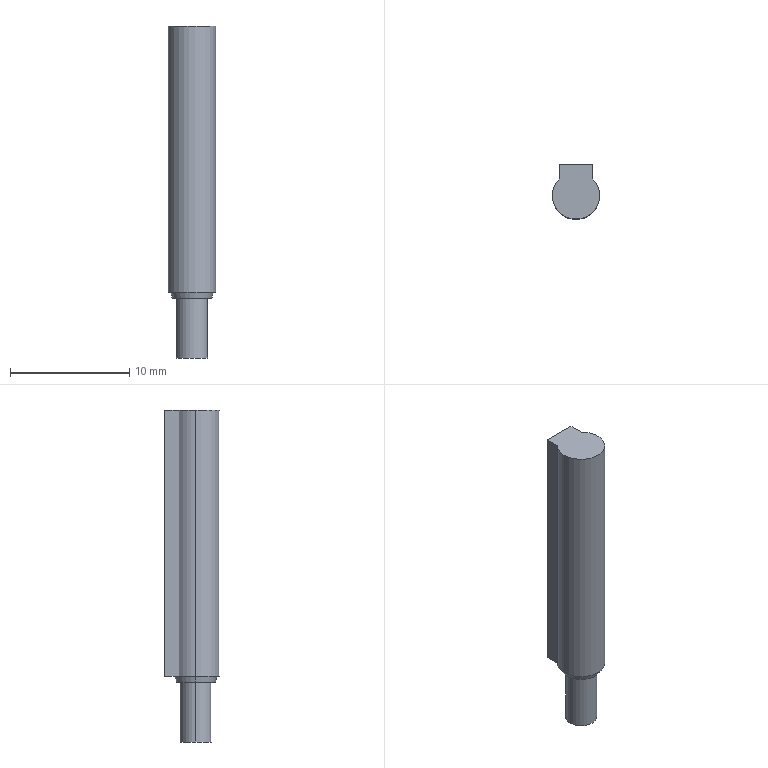Part | SolidWorks | features BaseBody 1 | 1 solid | 33 faces | box 3.95 x 4.575 x 27.8 mm | volume 349.99 mm3 | plane 18 | cylinder 13 | cone 2 | commonest cylinder face diameters 0.6 x4 3.95 x3 2 x2 2.5 x2 2.6 x2
STEP:
#1=CARTESIAN_POINT('',(-1.4,1.393,-22.3));
#2=VERTEX_POINT('',#1);
#3=CARTESIAN_POINT('',(-1.975,0.,-22.3));
#4=VERTEX_POINT('',#3);
#5=CARTESIAN_POINT('',(0.,0.,-22.3));
#6=DIRECTION('',(0.,0.,1.));
#7=DIRECTION('',(1.,0.,0.));
#8=AXIS2_PLACEMENT_3D('',#5,#6,#7);
#9=CIRCLE('',#8,1.975);
#10=EDGE_CURVE('',#2,#4,#9,.T.);
#11=ORIENTED_EDGE('',*,*,#10,.T.);
#12=CARTESIAN_POINT('',(-1.975,0.,0.));
#13=VERTEX_POINT('',#12);
#14=CARTESIAN_POINT('',(-1.975,0.,-22.3));
#15=DIRECTION('',(0.,0.,1.));
#16=VECTOR('',#15,1000.);
#17=LINE('',#14,#16);
#18=EDGE_CURVE('',#4,#13,#17,.T.);
#19=ORIENTED_EDGE('',*,*,#18,.T.);
#20=CARTESIAN_POINT('',(-1.4,1.393,0.));
#21=VERTEX_POINT('',#20);
#22=CARTESIAN_POINT('',(0.,0.,0.));
#23=DIRECTION('',(0.,0.,-1.));
#24=DIRECTION('',(1.,0.,0.));
#25=AXIS2_PLACEMENT_3D('',#22,#23,#24);
#26=CIRCLE('',#25,1.975);
#27=EDGE_CURVE('',#13,#21,#26,.T.);
#28=ORIENTED_EDGE('',*,*,#27,.T.);
#29=CARTESIAN_POINT('',(-1.4,1.393,-22.3));
#30=DIRECTION('',(0.,0.,-1.));
#31=VECTOR('',#30,1000.);
#32=LINE('',#29,#31);
#33=EDGE_CURVE('',#21,#2,#32,.T.);
#34=ORIENTED_EDGE('',*,*,#33,.T.);
#35=EDGE_LOOP('',(#11,#19,#28,#34));
#36=FACE_OUTER_BOUND('',#35,.T.);
#37=CARTESIAN_POINT('',(0.,0.,-22.3));
#38=DIRECTION('',(0.,0.,1.));
#39=DIRECTION('',(1.,0.,0.));
#40=AXIS2_PLACEMENT_3D('',#37,#38,#39);
#41=CYLINDRICAL_SURFACE('',#40,1.975);
#42=ADVANCED_FACE('',(#36),#41,.T.);
#43=ORIENTED_EDGE('',*,*,#18,.F.);
#44=CARTESIAN_POINT('',(1.975,0.,-22.3));
#45=VERTEX_POINT('',#44);
#46=CARTESIAN_POINT('',(0.,0.,-22.3));
#47=DIRECTION('',(0.,0.,1.));
#48=DIRECTION('',(1.,0.,0.));
#49=AXIS2_PLACEMENT_3D('',#46,#47,#48);
#50=CIRCLE('',#49,1.975);
#51=EDGE_CURVE('',#4,#45,#50,.T.);
#52=ORIENTED_EDGE('',*,*,#51,.T.);
#53=CARTESIAN_POINT('',(1.975,0.,0.));
#54=VERTEX_POINT('',#53);
#55=CARTESIAN_POINT('',(1.975,0.,-22.3));
#56=DIRECTION('',(0.,0.,1.));
#57=VECTOR('',#56,1000.);
#58=LINE('',#55,#57);
#59=EDGE_CURVE('',#45,#54,#58,.T.);
#60=ORIENTED_EDGE('',*,*,#59,.T.);
#61=CARTESIAN_POINT('',(0.,0.,0.));
#62=DIRECTION('',(0.,0.,-1.));
#63=DIRECTION('',(1.,0.,0.));
#64=AXIS2_PLACEMENT_3D('',#61,#62,#63);
#65=CIRCLE('',#64,1.975);
#66=EDGE_CURVE('',#54,#13,#65,.T.);
#67=ORIENTED_EDGE('',*,*,#66,.T.);
#68=EDGE_LOOP('',(#43,#52,#60,#67));
#69=FACE_OUTER_BOUND('',#68,.T.);
#70=CARTESIAN_POINT('',(0.,0.,-22.3));
#71=DIRECTION('',(0.,0.,1.));
#72=DIRECTION('',(1.,0.,0.));
#73=AXIS2_PLACEMENT_3D('',#70,#71,#72);
#74=CYLINDRICAL_SURFACE('',#73,1.975);
#75=ADVANCED_FACE('',(#69),#74,.T.);
#76=CARTESIAN_POINT('',(1.65,0.,-22.8));
#77=VERTEX_POINT('',#76);
#78=CARTESIAN_POINT('',(-1.65,0.,-22.8));
#79=VERTEX_POINT('',#78);
#80=CARTESIAN_POINT('',(0.,0.,-22.8));
#81=DIRECTION('',(0.,0.,1.));
#82=DIRECTION('',(1.,0.,0.));
#83=AXIS2_PLACEMENT_3D('',#80,#81,#82);
#84=CIRCLE('',#83,1.65);
#85=EDGE_CURVE('',#77,#79,#84,.T.);
#86=ORIENTED_EDGE('',*,*,#85,.T.);
#87=CARTESIAN_POINT('',(-1.784,0.,-22.3));
#88=VERTEX_POINT('',#87);
#89=CARTESIAN_POINT('',(-1.784,0.,-22.3));
#90=DIRECTION('',(-0.2588,0.,0.9659));
#91=VECTOR('',#90,1000.);
#92=LINE('',#89,#91);
#93=EDGE_CURVE('',#79,#88,#92,.T.);
#94=ORIENTED_EDGE('',*,*,#93,.T.);
#95=CARTESIAN_POINT('',(1.784,0.,-22.3));
#96=VERTEX_POINT('',#95);
#97=CARTESIAN_POINT('',(0.,0.,-22.3));
#98=DIRECTION('',(0.,0.,1.));
#99=DIRECTION('',(1.,0.,0.));
#100=AXIS2_PLACEMENT_3D('',#97,#98,#99);
#101=CIRCLE('',#100,1.784);
#102=EDGE_CURVE('',#96,#88,#101,.T.);
#103=ORIENTED_EDGE('',*,*,#102,.F.);
#104=CARTESIAN_POINT('',(1.784,0.,-22.3));
#105=DIRECTION('',(0.2588,0.,0.9659));
#106=VECTOR('',#105,1000.);
#107=LINE('',#104,#106);
#108=EDGE_CURVE('',#77,#96,#107,.T.);
#109=ORIENTED_EDGE('',*,*,#108,.F.);
#110=EDGE_LOOP('',(#86,#94,#103,#109));
#111=FACE_OUTER_BOUND('',#110,.T.);
#112=CARTESIAN_POINT('',(0.,0.,-22.3));
#113=DIRECTION('',(0.,0.,1.));
#114=DIRECTION('',(1.,0.,0.));
#115=AXIS2_PLACEMENT_3D('',#112,#113,#114);
#116=CONICAL_SURFACE('',#115,1.784,0.2618);
#117=ADVANCED_FACE('',(#111),#116,.T.);
#118=CARTESIAN_POINT('',(0.,1.1,-3.25));
#119=VERTEX_POINT('',#118);
#120=CARTESIAN_POINT('',(0.,1.1,-0.75));
#121=VERTEX_POINT('',#120);
#122=CARTESIAN_POINT('',(0.,1.1,-2.));
#123=DIRECTION('',(0.,1.,0.));
#124=DIRECTION('',(0.,0.,1.));
#125=AXIS2_PLACEMENT_3D('',#122,#123,#124);
#126=CIRCLE('',#125,1.25);
#127=EDGE_CURVE('',#119,#121,#126,.T.);
#128=ORIENTED_EDGE('',*,*,#127,.F.);
#129=CARTESIAN_POINT('',(0.,2.6,-3.25));
#130=VERTEX_POINT('',#129);
#131=CARTESIAN_POINT('',(0.,1.1,-3.25));
#132=DIRECTION('',(0.,1.,0.));
#133=VECTOR('',#132,1000.);
#134=LINE('',#131,#133);
#135=EDGE_CURVE('',#119,#130,#134,.T.);
#136=ORIENTED_EDGE('',*,*,#135,.T.);
#137=CARTESIAN_POINT('',(0.,2.6,-0.75));
#138=VERTEX_POINT('',#137);
#139=CARTESIAN_POINT('',(0.,2.6,-2.));
#140=DIRECTION('',(0.,1.,0.));
#141=DIRECTION('',(0.,0.,1.));
#142=AXIS2_PLACEMENT_3D('',#139,#140,#141);
#143=CIRCLE('',#142,1.25);
#144=EDGE_CURVE('',#130,#138,#143,.T.);
#145=ORIENTED_EDGE('',*,*,#144,.T.);
#146=CARTESIAN_POINT('',(0.,1.1,-0.75));
#147=DIRECTION('',(0.,1.,0.));
#148=VECTOR('',#147,1000.);
#149=LINE('',#146,#148);
#150=EDGE_CURVE('',#121,#138,#149,.T.);
#151=ORIENTED_EDGE('',*,*,#150,.F.);
#152=EDGE_LOOP('',(#128,#136,#145,#151));
#153=FACE_OUTER_BOUND('',#152,.T.);
#154=CARTESIAN_POINT('',(0.,1.1,-2.));
#155=DIRECTION('',(0.,1.,0.));
#156=DIRECTION('',(0.,0.,1.));
#157=AXIS2_PLACEMENT_3D('',#154,#155,#156);
#158=CYLINDRICAL_SURFACE('',#157,1.25);
#159=ADVANCED_FACE('',(#153),#158,.F.);
#160=CARTESIAN_POINT('',(1.3,0.,-27.8));
#161=VERTEX_POINT('',#160);
#162=CARTESIAN_POINT('',(-1.3,0.,-27.8));
#163=VERTEX_POINT('',#162);
#164=CARTESIAN_POINT('',(0.,0.,-27.8));
#165=DIRECTION('',(0.,0.,1.));
#166=DIRECTION('',(1.,0.,0.));
#167=AXIS2_PLACEMENT_3D('',#164,#165,#166);
#168=CIRCLE('',#167,1.3);
#169=EDGE_CURVE('',#161,#163,#168,.T.);
#170=ORIENTED_EDGE('',*,*,#169,.T.);
#171=CARTESIAN_POINT('',(-1.3,0.,-22.8));
#172=VERTEX_POINT('',#171);
#173=CARTESIAN_POINT('',(-1.3,0.,-27.8));
#174=DIRECTION('',(0.,0.,1.));
#175=VECTOR('',#174,1000.);
#176=LINE('',#173,#175);
#177=EDGE_CURVE('',#163,#172,#176,.T.);
#178=ORIENTED_EDGE('',*,*,#177,.T.);
#179=CARTESIAN_POINT('',(1.3,0.,-22.8));
#180=VERTEX_POINT('',#179);
#181=CARTESIAN_POINT('',(0.,0.,-22.8));
#182=DIRECTION('',(0.,0.,-1.));
#183=DIRECTION('',(1.,0.,0.));
#184=AXIS2_PLACEMENT_3D('',#181,#182,#183);
#185=CIRCLE('',#184,1.3);
#186=EDGE_CURVE('',#172,#180,#185,.T.);
#187=ORIENTED_EDGE('',*,*,#186,.T.);
#188=CARTESIAN_POINT('',(1.3,0.,-27.8));
#189=DIRECTION('',(0.,0.,1.));
#190=VECTOR('',#189,1000.);
#191=LINE('',#188,#190);
#192=EDGE_CURVE('',#161,#180,#191,.T.);
#193=ORIENTED_EDGE('',*,*,#192,.F.);
#194=EDGE_LOOP('',(#170,#178,#187,#193));
#195=FACE_OUTER_BOUND('',#194,.T.);
#196=CARTESIAN_POINT('',(0.,0.,-27.8));
#197=DIRECTION('',(0.,0.,1.));
#198=DIRECTION('',(1.,0.,0.));
#199=AXIS2_PLACEMENT_3D('',#196,#197,#198);
#200=CYLINDRICAL_SURFACE('',#199,1.3);
#201=ADVANCED_FACE('',(#195),#200,.T.);
#202=CARTESIAN_POINT('',(0.,1.1,-3.));
#203=VERTEX_POINT('',#202);
#204=CARTESIAN_POINT('',(0.,1.1,-1.));
#205=VERTEX_POINT('',#204);
#206=CARTESIAN_POINT('',(0.,1.1,-2.));
#207=DIRECTION('',(0.,-1.,0.));
#208=DIRECTION('',(0.,0.,1.));
#209=AXIS2_PLACEMENT_3D('',#206,#207,#208);
#210=CIRCLE('',#209,1.);
#211=EDGE_CURVE('',#203,#205,#210,.T.);
#212=ORIENTED_EDGE('',*,*,#211,.F.);
#213=CARTESIAN_POINT('',(0.,2.6,-3.));
#214=VERTEX_POINT('',#213);
#215=CARTESIAN_POINT('',(0.,1.1,-3.));
#216=DIRECTION('',(0.,1.,0.));
#217=VECTOR('',#216,1000.);
#218=LINE('',#215,#217);
#219=EDGE_CURVE('',#203,#214,#218,.T.);
#220=ORIENTED_EDGE('',*,*,#219,.T.);
#221=CARTESIAN_POINT('',(0.8867,2.6,-1.538));
#222=VERTEX_POINT('',#221);
#223=CARTESIAN_POINT('',(0.,2.6,-2.));
#224=DIRECTION('',(0.,-1.,0.));
#225=DIRECTION('',(0.,0.,1.));
#226=AXIS2_PLACEMENT_3D('',#223,#224,#225);
#227=CIRCLE('',#226,1.);
#228=EDGE_CURVE('',#214,#222,#227,.T.);
#229=ORIENTED_EDGE('',*,*,#228,.T.);
#230=CARTESIAN_POINT('',(0.8867,1.6,-1.538));
#231=VERTEX_POINT('',#230);
#232=CARTESIAN_POINT('',(0.8867,1.6,-1.538));
#233=DIRECTION('',(0.,-1.,0.));
#234=VECTOR('',#233,1000.);
#235=LINE('',#232,#234);
#236=EDGE_CURVE('',#222,#231,#235,.T.);
#237=ORIENTED_EDGE('',*,*,#236,.T.);
#238=CARTESIAN_POINT('',(0.4624,1.6,-1.113));
#239=VERTEX_POINT('',#238);
#240=CARTESIAN_POINT('',(0.,1.6,-2.));
#241=DIRECTION('',(0.,1.,0.));
#242=DIRECTION('',(0.,0.,1.));
#243=AXIS2_PLACEMENT_3D('',#240,#241,#242);
#244=CIRCLE('',#243,1.);
#245=EDGE_CURVE('',#239,#231,#244,.T.);
#246=ORIENTED_EDGE('',*,*,#245,.F.);
#247=CARTESIAN_POINT('',(0.4624,2.6,-1.113));
#248=VERTEX_POINT('',#247);
#249=CARTESIAN_POINT('',(0.4624,1.6,-1.113));
#250=DIRECTION('',(0.,1.,0.));
#251=VECTOR('',#250,1000.);
#252=LINE('',#249,#251);
#253=EDGE_CURVE('',#239,#248,#252,.T.);
#254=ORIENTED_EDGE('',*,*,#253,.T.);
#255=CARTESIAN_POINT('',(0.,2.6,-1.));
#256=VERTEX_POINT('',#255);
#257=CARTESIAN_POINT('',(0.,2.6,-2.));
#258=DIRECTION('',(0.,-1.,0.));
#259=DIRECTION('',(0.,0.,1.));
#260=AXIS2_PLACEMENT_3D('',#257,#258,#259);
#261=CIRCLE('',#260,1.);
#262=EDGE_CURVE('',#248,#256,#261,.T.);
#263=ORIENTED_EDGE('',*,*,#262,.T.);
#264=CARTESIAN_POINT('',(0.,1.1,-1.));
#265=DIRECTION('',(0.,1.,0.));
#266=VECTOR('',#265,1000.);
#267=LINE('',#264,#266);
#268=EDGE_CURVE('',#205,#256,#267,.T.);
#269=ORIENTED_EDGE('',*,*,#268,.F.);
#270=EDGE_LOOP('',(#212,#220,#229,#237,#246,#254,#263,#269));
#271=FACE_OUTER_BOUND('',#270,.T.);
#272=CARTESIAN_POINT('',(0.,1.1,-2.));
#273=DIRECTION('',(0.,1.,0.));
#274=DIRECTION('',(0.,0.,1.));
#275=AXIS2_PLACEMENT_3D('',#272,#273,#274);
#276=CYLINDRICAL_SURFACE('',#275,1.);
#277=ADVANCED_FACE('',(#271),#276,.T.);
#278=ORIENTED_EDGE('',*,*,#59,.F.);
#279=CARTESIAN_POINT('',(1.4,1.393,-22.3));
#280=VERTEX_POINT('',#279);
#281=CARTESIAN_POINT('',(0.,0.,-22.3));
#282=DIRECTION('',(0.,0.,1.));
#283=DIRECTION('',(1.,0.,0.));
#284=AXIS2_PLACEMENT_3D('',#281,#282,#283);
#285=CIRCLE('',#284,1.975);
#286=EDGE_CURVE('',#45,#280,#285,.T.);
#287=ORIENTED_EDGE('',*,*,#286,.T.);
#288=CARTESIAN_POINT('',(1.4,1.393,0.));
#289=VERTEX_POINT('',#288);
#290=CARTESIAN_POINT('',(1.4,1.393,-22.3));
#291=DIRECTION('',(0.,0.,1.));
#292=VECTOR('',#291,1000.);
#293=LINE('',#290,#292);
#294=EDGE_CURVE('',#280,#289,#293,.T.);
#295=ORIENTED_EDGE('',*,*,#294,.T.);
#296=CARTESIAN_POINT('',(0.,0.,0.));
#297=DIRECTION('',(0.,0.,-1.));
#298=DIRECTION('',(1.,0.,0.));
#299=AXIS2_PLACEMENT_3D('',#296,#297,#298);
#300=CIRCLE('',#299,1.975);
#301=EDGE_CURVE('',#289,#54,#300,.T.);
#302=ORIENTED_EDGE('',*,*,#301,.T.);
#303=EDGE_LOOP('',(#278,#287,#295,#302));
#304=FACE_OUTER_BOUND('',#303,.T.);
#305=CARTESIAN_POINT('',(0.,0.,-22.3));
#306=DIRECTION('',(0.,0.,1.));
#307=DIRECTION('',(1.,0.,0.));
#308=AXIS2_PLACEMENT_3D('',#305,#306,#307);
#309=CYLINDRICAL_SURFACE('',#308,1.975);
#310=ADVANCED_FACE('',(#304),#309,.T.);
#311=ORIENTED_EDGE('',*,*,#294,.F.);
#312=CARTESIAN_POINT('',(1.4,2.6,-22.3));
#313=VERTEX_POINT('',#312);
#314=CARTESIAN_POINT('',(1.4,2.6,-22.3));
#315=DIRECTION('',(0.,-1.,0.));
#316=VECTOR('',#315,1000.);
#317=LINE('',#314,#316);
#318=EDGE_CURVE('',#313,#280,#317,.T.);
#319=ORIENTED_EDGE('',*,*,#318,.F.);
#320=CARTESIAN_POINT('',(1.4,2.6,0.));
#321=VERTEX_POINT('',#320);
#322=CARTESIAN_POINT('',(1.4,2.6,-22.3));
#323=DIRECTION('',(0.,0.,-1.));
#324=VECTOR('',#323,1000.);
#325=LINE('',#322,#324);
#326=EDGE_CURVE('',#321,#313,#325,.T.);
#327=ORIENTED_EDGE('',*,*,#326,.F.);
#328=CARTESIAN_POINT('',(1.4,2.6,0.));
#329=DIRECTION('',(0.,1.,0.));
#330=VECTOR('',#329,1000.);
#331=LINE('',#328,#330);
#332=EDGE_CURVE('',#289,#321,#331,.T.);
#333=ORIENTED_EDGE('',*,*,#332,.F.);
#334=EDGE_LOOP('',(#311,#319,#327,#333));
#335=FACE_OUTER_BOUND('',#334,.T.);
#336=CARTESIAN_POINT('',(1.4,2.6,-22.3));
#337=DIRECTION('',(-1.,0.,0.));
#338=DIRECTION('',(0.,0.,1.));
#339=AXIS2_PLACEMENT_3D('',#336,#337,#338);
#340=PLANE('',#339);
#341=ADVANCED_FACE('',(#335),#340,.F.);
#342=CARTESIAN_POINT('',(-1.4,2.6,-22.3));
#343=VERTEX_POINT('',#342);
#344=CARTESIAN_POINT('',(-1.4,0.,-22.3));
#345=DIRECTION('',(0.,1.,0.));
#346=VECTOR('',#345,1000.);
#347=LINE('',#344,#346);
#348=EDGE_CURVE('',#2,#343,#347,.T.);
#349=ORIENTED_EDGE('',*,*,#348,.T.);
#350=CARTESIAN_POINT('',(0.,2.6,-22.3));
#351=DIRECTION('',(1.,0.,0.));
#352=VECTOR('',#351,1000.);
#353=LINE('',#350,#352);
#354=EDGE_CURVE('',#343,#313,#353,.T.);
#355=ORIENTED_EDGE('',*,*,#354,.T.);
#356=ORIENTED_EDGE('',*,*,#318,.T.);
#357=ORIENTED_EDGE('',*,*,#286,.F.);
#358=ORIENTED_EDGE('',*,*,#51,.F.);
#359=ORIENTED_EDGE('',*,*,#10,.F.);
#360=EDGE_LOOP('',(#349,#355,#356,#357,#358,#359));
#361=FACE_OUTER_BOUND('',#360,.T.);
#362=ORIENTED_EDGE('',*,*,#102,.T.);
#363=CARTESIAN_POINT('',(0.,0.,-22.3));
#364=DIRECTION('',(0.,0.,1.));
#365=DIRECTION('',(1.,0.,0.));
#366=AXIS2_PLACEMENT_3D('',#363,#364,#365);
#367=CIRCLE('',#366,1.784);
#368=EDGE_CURVE('',#88,#96,#367,.T.);
#369=ORIENTED_EDGE('',*,*,#368,.T.);
#370=EDGE_LOOP('',(#362,#369));
#371=FACE_BOUND('',#370,.T.);
#372=CARTESIAN_POINT('',(0.,0.,-22.3));
#373=DIRECTION('',(0.,0.,-1.));
#374=DIRECTION('',(-1.,0.,0.));
#375=AXIS2_PLACEMENT_3D('',#372,#373,#374);
#376=PLANE('',#375);
#377=ADVANCED_FACE('',(#361,#371),#376,.T.);
#378=CARTESIAN_POINT('',(-1.4,2.6,0.));
#379=VERTEX_POINT('',#378);
#380=CARTESIAN_POINT('',(-1.4,2.6,-22.3));
#381=DIRECTION('',(0.,0.,1.));
#382=VECTOR('',#381,1000.);
#383=LINE('',#380,#382);
#384=EDGE_CURVE('',#343,#379,#383,.T.);
#385=ORIENTED_EDGE('',*,*,#384,.F.);
#386=ORIENTED_EDGE('',*,*,#348,.F.);
#387=ORIENTED_EDGE('',*,*,#33,.F.);
#388=CARTESIAN_POINT('',(-1.4,1.393,0.));
#389=DIRECTION('',(0.,-1.,0.));
#390=VECTOR('',#389,1000.);
#391=LINE('',#388,#390);
#392=EDGE_CURVE('',#379,#21,#391,.T.);
#393=ORIENTED_EDGE('',*,*,#392,.F.);
#394=EDGE_LOOP('',(#385,#386,#387,#393));
#395=FACE_OUTER_BOUND('',#394,.T.);
#396=CARTESIAN_POINT('',(-1.4,1.393,-22.3));
#397=DIRECTION('',(1.,0.,0.));
#398=DIRECTION('',(0.,0.,-1.));
#399=AXIS2_PLACEMENT_3D('',#396,#397,#398);
#400=PLANE('',#399);
#401=ADVANCED_FACE('',(#395),#400,.F.);
#402=CARTESIAN_POINT('',(0.,2.6,0.));
#403=DIRECTION('',(1.,0.,0.));
#404=VECTOR('',#403,1000.);
#405=LINE('',#402,#404);
#406=EDGE_CURVE('',#379,#321,#405,.T.);
#407=ORIENTED_EDGE('',*,*,#406,.F.);
#408=ORIENTED_EDGE('',*,*,#392,.T.);
#409=ORIENTED_EDGE('',*,*,#27,.F.);
#410=ORIENTED_EDGE('',*,*,#66,.F.);
#411=ORIENTED_EDGE('',*,*,#301,.F.);
#412=ORIENTED_EDGE('',*,*,#332,.T.);
#413=EDGE_LOOP('',(#407,#408,#409,#410,#411,#412));
#414=FACE_OUTER_BOUND('',#413,.T.);
#415=CARTESIAN_POINT('',(0.,0.,0.));
#416=DIRECTION('',(0.,0.,-1.));
#417=DIRECTION('',(-1.,0.,0.));
#418=AXIS2_PLACEMENT_3D('',#415,#416,#417);
#419=PLANE('',#418);
#420=ADVANCED_FACE('',(#414),#419,.F.);
#421=ORIENTED_EDGE('',*,*,#326,.T.);
#422=ORIENTED_EDGE('',*,*,#354,.F.);
#423=ORIENTED_EDGE('',*,*,#384,.T.);
#424=ORIENTED_EDGE('',*,*,#406,.T.);
#425=EDGE_LOOP('',(#421,#422,#423,#424));
#426=FACE_OUTER_BOUND('',#425,.T.);
#427=CARTESIAN_POINT('',(0.,2.6,-2.));
#428=DIRECTION('',(0.,1.,0.));
#429=DIRECTION('',(0.,0.,1.));
#430=AXIS2_PLACEMENT_3D('',#427,#428,#429);
#431=CIRCLE('',#430,1.25);
#432=EDGE_CURVE('',#138,#130,#431,.T.);
#433=ORIENTED_EDGE('',*,*,#432,.F.);
#434=ORIENTED_EDGE('',*,*,#144,.F.);
#435=EDGE_LOOP('',(#433,#434));
#436=FACE_BOUND('',#435,.T.);
#437=CARTESIAN_POINT('',(-0.8,2.6,-8.3));
#438=VERTEX_POINT('',#437);
#439=CARTESIAN_POINT('',(-0.5,2.6,-8.));
#440=VERTEX_POINT('',#439);
#441=CARTESIAN_POINT('',(-0.5,2.6,-8.3));
#442=DIRECTION('',(0.,1.,0.));
#443=DIRECTION('',(0.,0.,1.));
#444=AXIS2_PLACEMENT_3D('',#441,#442,#443);
#445=CIRCLE('',#444,0.3);
#446=EDGE_CURVE('',#438,#440,#445,.T.);
#447=ORIENTED_EDGE('',*,*,#446,.F.);
#448=CARTESIAN_POINT('',(-0.8,2.6,-10.7));
#449=VERTEX_POINT('',#448);
#450=CARTESIAN_POINT('',(-0.8,2.6,-22.3));
#451=DIRECTION('',(0.,0.,1.));
#452=VECTOR('',#451,1000.);
#453=LINE('',#450,#452);
#454=EDGE_CURVE('',#449,#438,#453,.T.);
#455=ORIENTED_EDGE('',*,*,#454,.F.);
#456=CARTESIAN_POINT('',(-0.5,2.6,-11.));
#457=VERTEX_POINT('',#456);
#458=CARTESIAN_POINT('',(-0.5,2.6,-10.7));
#459=DIRECTION('',(0.,1.,0.));
#460=DIRECTION('',(0.,0.,1.));
#461=AXIS2_PLACEMENT_3D('',#458,#459,#460);
#462=CIRCLE('',#461,0.3);
#463=EDGE_CURVE('',#457,#449,#462,.T.);
#464=ORIENTED_EDGE('',*,*,#463,.F.);
#465=CARTESIAN_POINT('',(0.5,2.6,-11.));
#466=VERTEX_POINT('',#465);
#467=CARTESIAN_POINT('',(-1.4,2.6,-11.));
#468=DIRECTION('',(-1.,0.,0.));
#469=VECTOR('',#468,1000.);
#470=LINE('',#467,#469);
#471=EDGE_CURVE('',#466,#457,#470,.T.);
#472=ORIENTED_EDGE('',*,*,#471,.F.);
#473=CARTESIAN_POINT('',(0.8,2.6,-10.7));
#474=VERTEX_POINT('',#473);
#475=CARTESIAN_POINT('',(0.5,2.6,-10.7));
#476=DIRECTION('',(0.,1.,0.));
#477=DIRECTION('',(0.,0.,1.));
#478=AXIS2_PLACEMENT_3D('',#475,#476,#477);
#479=CIRCLE('',#478,0.3);
#480=EDGE_CURVE('',#474,#466,#479,.T.);
#481=ORIENTED_EDGE('',*,*,#480,.F.);
#482=CARTESIAN_POINT('',(0.8,2.6,-8.3));
#483=VERTEX_POINT('',#482);
#484=CARTESIAN_POINT('',(0.8,2.6,-22.3));
#485=DIRECTION('',(0.,0.,-1.));
#486=VECTOR('',#485,1000.);
#487=LINE('',#484,#486);
#488=EDGE_CURVE('',#483,#474,#487,.T.);
#489=ORIENTED_EDGE('',*,*,#488,.F.);
#490=CARTESIAN_POINT('',(0.5,2.6,-8.));
#491=VERTEX_POINT('',#490);
#492=CARTESIAN_POINT('',(0.5,2.6,-8.3));
#493=DIRECTION('',(0.,1.,0.));
#494=DIRECTION('',(0.,0.,1.));
#495=AXIS2_PLACEMENT_3D('',#492,#493,#494);
#496=CIRCLE('',#495,0.3);
#497=EDGE_CURVE('',#491,#483,#496,.T.);
#498=ORIENTED_EDGE('',*,*,#497,.F.);
#499=CARTESIAN_POINT('',(-1.4,2.6,-8.));
#500=DIRECTION('',(1.,0.,0.));
#501=VECTOR('',#500,1000.);
#502=LINE('',#499,#501);
#503=EDGE_CURVE('',#440,#491,#502,.T.);
#504=ORIENTED_EDGE('',*,*,#503,.F.);
#505=EDGE_LOOP('',(#447,#455,#464,#472,#481,#489,#498,#504));
#506=FACE_BOUND('',#505,.T.);
#507=CARTESIAN_POINT('',(-1.4,2.6,-22.3));
#508=DIRECTION('',(0.,-1.,0.));
#509=DIRECTION('',(0.,0.,-1.));
#510=AXIS2_PLACEMENT_3D('',#507,#508,#509);
#511=PLANE('',#510);
#512=ADVANCED_FACE('',(#426,#436,#506),#511,.F.);
#513=ORIENTED_EDGE('',*,*,#93,.F.);
#514=CARTESIAN_POINT('',(0.,0.,-22.8));
#515=DIRECTION('',(0.,0.,1.));
#516=DIRECTION('',(1.,0.,0.));
#517=AXIS2_PLACEMENT_3D('',#514,#515,#516);
#518=CIRCLE('',#517,1.65);
#519=EDGE_CURVE('',#79,#77,#518,.T.);
#520=ORIENTED_EDGE('',*,*,#519,.T.);
#521=ORIENTED_EDGE('',*,*,#108,.T.);
#522=ORIENTED_EDGE('',*,*,#368,.F.);
#523=EDGE_LOOP('',(#513,#520,#521,#522));
#524=FACE_OUTER_BOUND('',#523,.T.);
#525=CARTESIAN_POINT('',(0.,0.,-22.3));
#526=DIRECTION('',(0.,0.,1.));
#527=DIRECTION('',(1.,0.,0.));
#528=AXIS2_PLACEMENT_3D('',#525,#526,#527);
#529=CONICAL_SURFACE('',#528,1.784,0.2618);
#530=ADVANCED_FACE('',(#524),#529,.T.);
#531=ORIENTED_EDGE('',*,*,#135,.F.);
#532=CARTESIAN_POINT('',(0.,1.1,-2.));
#533=DIRECTION('',(0.,1.,0.));
#534=DIRECTION('',(0.,0.,1.));
#535=AXIS2_PLACEMENT_3D('',#532,#533,#534);
#536=CIRCLE('',#535,1.25);
#537=EDGE_CURVE('',#121,#119,#536,.T.);
#538=ORIENTED_EDGE('',*,*,#537,.F.);
#539=ORIENTED_EDGE('',*,*,#150,.T.);
#540=ORIENTED_EDGE('',*,*,#432,.T.);
#541=EDGE_LOOP('',(#531,#538,#539,#540));
#542=FACE_OUTER_BOUND('',#541,.T.);
#543=CARTESIAN_POINT('',(0.,1.1,-2.));
#544=DIRECTION('',(0.,1.,0.));
#545=DIRECTION('',(0.,0.,1.));
#546=AXIS2_PLACEMENT_3D('',#543,#544,#545);
#547=CYLINDRICAL_SURFACE('',#546,1.25);
#548=ADVANCED_FACE('',(#542),#547,.F.);
#549=CARTESIAN_POINT('',(0.5,2.4,-8.));
#550=VERTEX_POINT('',#549);
#551=CARTESIAN_POINT('',(0.5,2.4,-8.));
#552=DIRECTION('',(0.,1.,0.));
#553=VECTOR('',#552,1000.);
#554=LINE('',#551,#553);
#555=EDGE_CURVE('',#550,#491,#554,.T.);
#556=ORIENTED_EDGE('',*,*,#555,.F.);
#557=CARTESIAN_POINT('',(-0.5,2.4,-8.));
#558=VERTEX_POINT('',#557);
#559=CARTESIAN_POINT('',(-0.5,2.4,-8.));
#560=DIRECTION('',(1.,0.,0.));
#561=VECTOR('',#560,1000.);
#562=LINE('',#559,#561);
#563=EDGE_CURVE('',#558,#550,#562,.T.);
#564=ORIENTED_EDGE('',*,*,#563,.F.);
#565=CARTESIAN_POINT('',(-0.5,2.4,-8.));
#566=DIRECTION('',(0.,-1.,0.));
#567=VECTOR('',#566,1000.);
#568=LINE('',#565,#567);
#569=EDGE_CURVE('',#440,#558,#568,.T.);
#570=ORIENTED_EDGE('',*,*,#569,.F.);
#571=ORIENTED_EDGE('',*,*,#503,.T.);
#572=EDGE_LOOP('',(#556,#564,#570,#571));
#573=FACE_OUTER_BOUND('',#572,.T.);
#574=CARTESIAN_POINT('',(-0.5,2.4,-8.));
#575=DIRECTION('',(0.,0.,1.));
#576=DIRECTION('',(1.,0.,0.));
#577=AXIS2_PLACEMENT_3D('',#574,#575,#576);
#578=PLANE('',#577);
#579=ADVANCED_FACE('',(#573),#578,.F.);
#580=ORIENTED_EDGE('',*,*,#569,.T.);
#581=CARTESIAN_POINT('',(-0.8,2.4,-8.3));
#582=VERTEX_POINT('',#581);
#583=CARTESIAN_POINT('',(-0.5,2.4,-8.3));
#584=DIRECTION('',(0.,1.,0.));
#585=DIRECTION('',(0.,0.,1.));
#586=AXIS2_PLACEMENT_3D('',#583,#584,#585);
#587=CIRCLE('',#586,0.3);
#588=EDGE_CURVE('',#582,#558,#587,.T.);
#589=ORIENTED_EDGE('',*,*,#588,.F.);
#590=CARTESIAN_POINT('',(-0.8,2.4,-8.3));
#591=DIRECTION('',(0.,-1.,0.));
#592=VECTOR('',#591,1000.);
#593=LINE('',#590,#592);
#594=EDGE_CURVE('',#438,#582,#593,.T.);
#595=ORIENTED_EDGE('',*,*,#594,.F.);
#596=ORIENTED_EDGE('',*,*,#446,.T.);
#597=EDGE_LOOP('',(#580,#589,#595,#596));
#598=FACE_OUTER_BOUND('',#597,.T.);
#599=CARTESIAN_POINT('',(-0.5,2.4,-8.3));
#600=DIRECTION('',(0.,1.,0.));
#601=DIRECTION('',(0.,0.,1.));
#602=AXIS2_PLACEMENT_3D('',#599,#600,#601);
#603=CYLINDRICAL_SURFACE('',#602,0.3);
#604=ADVANCED_FACE('',(#598),#603,.F.);
#605=ORIENTED_EDGE('',*,*,#594,.T.);
#606=CARTESIAN_POINT('',(-0.8,2.4,-10.7));
#607=VERTEX_POINT('',#606);
#608=CARTESIAN_POINT('',(-0.8,2.4,-10.7));
#609=DIRECTION('',(0.,0.,1.));
#610=VECTOR('',#609,1000.);
#611=LINE('',#608,#610);
#612=EDGE_CURVE('',#607,#582,#611,.T.);
#613=ORIENTED_EDGE('',*,*,#612,.F.);
#614=CARTESIAN_POINT('',(-0.8,2.4,-10.7));
#615=DIRECTION('',(0.,-1.,0.));
#616=VECTOR('',#615,1000.);
#617=LINE('',#614,#616);
#618=EDGE_CURVE('',#449,#607,#617,.T.);
#619=ORIENTED_EDGE('',*,*,#618,.F.);
#620=ORIENTED_EDGE('',*,*,#454,.T.);
#621=EDGE_LOOP('',(#605,#613,#619,#620));
#622=FACE_OUTER_BOUND('',#621,.T.);
#623=CARTESIAN_POINT('',(-0.8,2.4,-10.7));
#624=DIRECTION('',(-1.,0.,0.));
#625=DIRECTION('',(0.,0.,1.));
#626=AXIS2_PLACEMENT_3D('',#623,#624,#625);
#627=PLANE('',#626);
#628=ADVANCED_FACE('',(#622),#627,.F.);
#629=ORIENTED_EDGE('',*,*,#618,.T.);
#630=CARTESIAN_POINT('',(-0.5,2.4,-11.));
#631=VERTEX_POINT('',#630);
#632=CARTESIAN_POINT('',(-0.5,2.4,-10.7));
#633=DIRECTION('',(0.,1.,0.));
#634=DIRECTION('',(0.,0.,1.));
#635=AXIS2_PLACEMENT_3D('',#632,#633,#634);
#636=CIRCLE('',#635,0.3);
#637=EDGE_CURVE('',#631,#607,#636,.T.);
#638=ORIENTED_EDGE('',*,*,#637,.F.);
#639=CARTESIAN_POINT('',(-0.5,2.4,-11.));
#640=DIRECTION('',(0.,-1.,0.));
#641=VECTOR('',#640,1000.);
#642=LINE('',#639,#641);
#643=EDGE_CURVE('',#457,#631,#642,.T.);
#644=ORIENTED_EDGE('',*,*,#643,.F.);
#645=ORIENTED_EDGE('',*,*,#463,.T.);
#646=EDGE_LOOP('',(#629,#638,#644,#645));
#647=FACE_OUTER_BOUND('',#646,.T.);
#648=CARTESIAN_POINT('',(-0.5,2.4,-10.7));
#649=DIRECTION('',(0.,1.,0.));
#650=DIRECTION('',(0.,0.,1.));
#651=AXIS2_PLACEMENT_3D('',#648,#649,#650);
#652=CYLINDRICAL_SURFACE('',#651,0.3);
#653=ADVANCED_FACE('',(#647),#652,.F.);
#654=ORIENTED_EDGE('',*,*,#643,.T.);
#655=CARTESIAN_POINT('',(0.5,2.4,-11.));
#656=VERTEX_POINT('',#655);
#657=CARTESIAN_POINT('',(0.5,2.4,-11.));
#658=DIRECTION('',(-1.,0.,0.));
#659=VECTOR('',#658,1000.);
#660=LINE('',#657,#659);
#661=EDGE_CURVE('',#656,#631,#660,.T.);
#662=ORIENTED_EDGE('',*,*,#661,.F.);
#663=CARTESIAN_POINT('',(0.5,2.4,-11.));
#664=DIRECTION('',(0.,-1.,0.));
#665=VECTOR('',#664,1000.);
#666=LINE('',#663,#665);
#667=EDGE_CURVE('',#466,#656,#666,.T.);
#668=ORIENTED_EDGE('',*,*,#667,.F.);
#669=ORIENTED_EDGE('',*,*,#471,.T.);
#670=EDGE_LOOP('',(#654,#662,#668,#669));
#671=FACE_OUTER_BOUND('',#670,.T.);
#672=CARTESIAN_POINT('',(0.5,2.4,-11.));
#673=DIRECTION('',(0.,0.,-1.));
#674=DIRECTION('',(-1.,0.,0.));
#675=AXIS2_PLACEMENT_3D('',#672,#673,#674);
#676=PLANE('',#675);
#677=ADVANCED_FACE('',(#671),#676,.F.);
#678=ORIENTED_EDGE('',*,*,#667,.T.);
#679=CARTESIAN_POINT('',(0.8,2.4,-10.7));
#680=VERTEX_POINT('',#679);
#681=CARTESIAN_POINT('',(0.5,2.4,-10.7));
#682=DIRECTION('',(0.,1.,0.));
#683=DIRECTION('',(0.,0.,1.));
#684=AXIS2_PLACEMENT_3D('',#681,#682,#683);
#685=CIRCLE('',#684,0.3);
#686=EDGE_CURVE('',#680,#656,#685,.T.);
#687=ORIENTED_EDGE('',*,*,#686,.F.);
#688=CARTESIAN_POINT('',(0.8,2.4,-10.7));
#689=DIRECTION('',(0.,-1.,0.));
#690=VECTOR('',#689,1000.);
#691=LINE('',#688,#690);
#692=EDGE_CURVE('',#474,#680,#691,.T.);
#693=ORIENTED_EDGE('',*,*,#692,.F.);
#694=ORIENTED_EDGE('',*,*,#480,.T.);
#695=EDGE_LOOP('',(#678,#687,#693,#694));
#696=FACE_OUTER_BOUND('',#695,.T.);
#697=CARTESIAN_POINT('',(0.5,2.4,-10.7));
#698=DIRECTION('',(0.,1.,0.));
#699=DIRECTION('',(0.,0.,1.));
#700=AXIS2_PLACEMENT_3D('',#697,#698,#699);
#701=CYLINDRICAL_SURFACE('',#700,0.3);
#702=ADVANCED_FACE('',(#696),#701,.F.);
#703=ORIENTED_EDGE('',*,*,#692,.T.);
#704=CARTESIAN_POINT('',(0.8,2.4,-8.3));
#705=VERTEX_POINT('',#704);
#706=CARTESIAN_POINT('',(0.8,2.4,-8.3));
#707=DIRECTION('',(0.,0.,-1.));
#708=VECTOR('',#707,1000.);
#709=LINE('',#706,#708);
#710=EDGE_CURVE('',#705,#680,#709,.T.);
#711=ORIENTED_EDGE('',*,*,#710,.F.);
#712=CARTESIAN_POINT('',(0.8,2.4,-8.3));
#713=DIRECTION('',(0.,-1.,0.));
#714=VECTOR('',#713,1000.);
#715=LINE('',#712,#714);
#716=EDGE_CURVE('',#483,#705,#715,.T.);
#717=ORIENTED_EDGE('',*,*,#716,.F.);
#718=ORIENTED_EDGE('',*,*,#488,.T.);
#719=EDGE_LOOP('',(#703,#711,#717,#718));
#720=FACE_OUTER_BOUND('',#719,.T.);
#721=CARTESIAN_POINT('',(0.8,2.4,-8.3));
#722=DIRECTION('',(1.,0.,0.));
#723=DIRECTION('',(0.,0.,-1.));
#724=AXIS2_PLACEMENT_3D('',#721,#722,#723);
#725=PLANE('',#724);
#726=ADVANCED_FACE('',(#720),#725,.F.);
#727=ORIENTED_EDGE('',*,*,#716,.T.);
#728=CARTESIAN_POINT('',(0.5,2.4,-8.3));
#729=DIRECTION('',(0.,1.,0.));
#730=DIRECTION('',(0.,0.,1.));
#731=AXIS2_PLACEMENT_3D('',#728,#729,#730);
#732=CIRCLE('',#731,0.3);
#733=EDGE_CURVE('',#550,#705,#732,.T.);
#734=ORIENTED_EDGE('',*,*,#733,.F.);
#735=ORIENTED_EDGE('',*,*,#555,.T.);
#736=ORIENTED_EDGE('',*,*,#497,.T.);
#737=EDGE_LOOP('',(#727,#734,#735,#736));
#738=FACE_OUTER_BOUND('',#737,.T.);
#739=CARTESIAN_POINT('',(0.5,2.4,-8.3));
#740=DIRECTION('',(0.,1.,0.));
#741=DIRECTION('',(0.,0.,1.));
#742=AXIS2_PLACEMENT_3D('',#739,#740,#741);
#743=CYLINDRICAL_SURFACE('',#742,0.3);
#744=ADVANCED_FACE('',(#738),#743,.F.);
#745=ORIENTED_EDGE('',*,*,#85,.F.);
#746=ORIENTED_EDGE('',*,*,#519,.F.);
#747=EDGE_LOOP('',(#745,#746));
#748=FACE_OUTER_BOUND('',#747,.T.);
#749=CARTESIAN_POINT('',(0.,0.,-22.8));
#750=DIRECTION('',(0.,0.,-1.));
#751=DIRECTION('',(1.,0.,0.));
#752=AXIS2_PLACEMENT_3D('',#749,#750,#751);
#753=CIRCLE('',#752,1.3);
#754=EDGE_CURVE('',#180,#172,#753,.T.);
#755=ORIENTED_EDGE('',*,*,#754,.F.);
#756=ORIENTED_EDGE('',*,*,#186,.F.);
#757=EDGE_LOOP('',(#755,#756));
#758=FACE_BOUND('',#757,.T.);
#759=CARTESIAN_POINT('',(0.,1.65,-22.8));
#760=DIRECTION('',(0.,0.,1.));
#761=DIRECTION('',(1.,0.,0.));
#762=AXIS2_PLACEMENT_3D('',#759,#760,#761);
#763=PLANE('',#762);
#764=ADVANCED_FACE('',(#748,#758),#763,.F.);
#765=ORIENTED_EDGE('',*,*,#537,.T.);
#766=ORIENTED_EDGE('',*,*,#127,.T.);
#767=EDGE_LOOP('',(#765,#766));
#768=FACE_OUTER_BOUND('',#767,.T.);
#769=CARTESIAN_POINT('',(0.,1.1,-2.));
#770=DIRECTION('',(0.,-1.,0.));
#771=DIRECTION('',(0.,0.,1.));
#772=AXIS2_PLACEMENT_3D('',#769,#770,#771);
#773=CIRCLE('',#772,1.);
#774=EDGE_CURVE('',#205,#203,#773,.T.);
#775=ORIENTED_EDGE('',*,*,#774,.T.);
#776=ORIENTED_EDGE('',*,*,#211,.T.);
#777=EDGE_LOOP('',(#775,#776));
#778=FACE_BOUND('',#777,.T.);
#779=CARTESIAN_POINT('',(0.,1.1,-2.));
#780=DIRECTION('',(0.,1.,0.));
#781=DIRECTION('',(0.,0.,1.));
#782=AXIS2_PLACEMENT_3D('',#779,#780,#781);
#783=PLANE('',#782);
#784=ADVANCED_FACE('',(#768,#778),#783,.T.);
#785=ORIENTED_EDGE('',*,*,#637,.T.);
#786=ORIENTED_EDGE('',*,*,#612,.T.);
#787=ORIENTED_EDGE('',*,*,#588,.T.);
#788=ORIENTED_EDGE('',*,*,#563,.T.);
#789=ORIENTED_EDGE('',*,*,#733,.T.);
#790=ORIENTED_EDGE('',*,*,#710,.T.);
#791=ORIENTED_EDGE('',*,*,#686,.T.);
#792=ORIENTED_EDGE('',*,*,#661,.T.);
#793=EDGE_LOOP('',(#785,#786,#787,#788,#789,#790,#791,#792));
#794=FACE_OUTER_BOUND('',#793,.T.);
#795=CARTESIAN_POINT('',(-0.5,2.4,-8.3));
#796=DIRECTION('',(0.,1.,0.));
#797=DIRECTION('',(0.,0.,1.));
#798=AXIS2_PLACEMENT_3D('',#795,#796,#797);
#799=PLANE('',#798);
#800=ADVANCED_FACE('',(#794),#799,.T.);
#801=ORIENTED_EDGE('',*,*,#177,.F.);
#802=CARTESIAN_POINT('',(0.,0.,-27.8));
#803=DIRECTION('',(0.,0.,1.));
#804=DIRECTION('',(1.,0.,0.));
#805=AXIS2_PLACEMENT_3D('',#802,#803,#804);
#806=CIRCLE('',#805,1.3);
#807=EDGE_CURVE('',#163,#161,#806,.T.);
#808=ORIENTED_EDGE('',*,*,#807,.T.);
#809=ORIENTED_EDGE('',*,*,#192,.T.);
#810=ORIENTED_EDGE('',*,*,#754,.T.);
#811=EDGE_LOOP('',(#801,#808,#809,#810));
#812=FACE_OUTER_BOUND('',#811,.T.);
#813=CARTESIAN_POINT('',(0.,0.,-27.8));
#814=DIRECTION('',(0.,0.,1.));
#815=DIRECTION('',(1.,0.,0.));
#816=AXIS2_PLACEMENT_3D('',#813,#814,#815);
#817=CYLINDRICAL_SURFACE('',#816,1.3);
#818=ADVANCED_FACE('',(#812),#817,.T.);
#819=ORIENTED_EDGE('',*,*,#219,.F.);
#820=ORIENTED_EDGE('',*,*,#774,.F.);
#821=ORIENTED_EDGE('',*,*,#268,.T.);
#822=CARTESIAN_POINT('',(-0.8867,2.6,-2.462));
#823=VERTEX_POINT('',#822);
#824=CARTESIAN_POINT('',(0.,2.6,-2.));
#825=DIRECTION('',(0.,-1.,0.));
#826=DIRECTION('',(0.,0.,1.));
#827=AXIS2_PLACEMENT_3D('',#824,#825,#826);
#828=CIRCLE('',#827,1.);
#829=EDGE_CURVE('',#256,#823,#828,.T.);
#830=ORIENTED_EDGE('',*,*,#829,.T.);
#831=CARTESIAN_POINT('',(-0.8867,1.6,-2.462));
#832=VERTEX_POINT('',#831);
#833=CARTESIAN_POINT('',(-0.8867,1.6,-2.462));
#834=DIRECTION('',(0.,-1.,0.));
#835=VECTOR('',#834,1000.);
#836=LINE('',#833,#835);
#837=EDGE_CURVE('',#823,#832,#836,.T.);
#838=ORIENTED_EDGE('',*,*,#837,.T.);
#839=CARTESIAN_POINT('',(-0.4624,1.6,-2.887));
#840=VERTEX_POINT('',#839);
#841=CARTESIAN_POINT('',(0.,1.6,-2.));
#842=DIRECTION('',(0.,1.,0.));
#843=DIRECTION('',(0.,0.,1.));
#844=AXIS2_PLACEMENT_3D('',#841,#842,#843);
#845=CIRCLE('',#844,1.);
#846=EDGE_CURVE('',#840,#832,#845,.T.);
#847=ORIENTED_EDGE('',*,*,#846,.F.);
#848=CARTESIAN_POINT('',(-0.4624,2.6,-2.887));
#849=VERTEX_POINT('',#848);
#850=CARTESIAN_POINT('',(-0.4624,1.6,-2.887));
#851=DIRECTION('',(0.,1.,0.));
#852=VECTOR('',#851,1000.);
#853=LINE('',#850,#852);
#854=EDGE_CURVE('',#840,#849,#853,.T.);
#855=ORIENTED_EDGE('',*,*,#854,.T.);
#856=CARTESIAN_POINT('',(0.,2.6,-2.));
#857=DIRECTION('',(0.,-1.,0.));
#858=DIRECTION('',(0.,0.,1.));
#859=AXIS2_PLACEMENT_3D('',#856,#857,#858);
#860=CIRCLE('',#859,1.);
#861=EDGE_CURVE('',#849,#214,#860,.T.);
#862=ORIENTED_EDGE('',*,*,#861,.T.);
#863=EDGE_LOOP('',(#819,#820,#821,#830,#838,#847,#855,#862));
#864=FACE_OUTER_BOUND('',#863,.T.);
#865=CARTESIAN_POINT('',(0.,1.1,-2.));
#866=DIRECTION('',(0.,1.,0.));
#867=DIRECTION('',(0.,0.,1.));
#868=AXIS2_PLACEMENT_3D('',#865,#866,#867);
#869=CYLINDRICAL_SURFACE('',#868,1.);
#870=ADVANCED_FACE('',(#864),#869,.T.);
#871=ORIENTED_EDGE('',*,*,#169,.F.);
#872=ORIENTED_EDGE('',*,*,#807,.F.);
#873=EDGE_LOOP('',(#871,#872));
#874=FACE_OUTER_BOUND('',#873,.T.);
#875=CARTESIAN_POINT('',(0.,0.,-27.8));
#876=DIRECTION('',(0.,0.,-1.));
#877=DIRECTION('',(-1.,0.,0.));
#878=AXIS2_PLACEMENT_3D('',#875,#876,#877);
#879=PLANE('',#878);
#880=ADVANCED_FACE('',(#874),#879,.T.);
#881=CARTESIAN_POINT('',(-0.8867,2.6,-2.462));
#882=DIRECTION('',(0.7071,0.,0.7071));
#883=VECTOR('',#882,1000.);
#884=LINE('',#881,#883);
#885=EDGE_CURVE('',#823,#248,#884,.T.);
#886=ORIENTED_EDGE('',*,*,#885,.F.);
#887=ORIENTED_EDGE('',*,*,#829,.F.);
#888=ORIENTED_EDGE('',*,*,#262,.F.);
#889=EDGE_LOOP('',(#886,#887,#888));
#890=FACE_OUTER_BOUND('',#889,.T.);
#891=CARTESIAN_POINT('',(-1.4,2.6,-22.3));
#892=DIRECTION('',(0.,-1.,0.));
#893=DIRECTION('',(0.,0.,-1.));
#894=AXIS2_PLACEMENT_3D('',#891,#892,#893);
#895=PLANE('',#894);
#896=ADVANCED_FACE('',(#890),#895,.F.);
#897=CARTESIAN_POINT('',(0.8867,2.6,-1.538));
#898=DIRECTION('',(-0.7071,0.,-0.7071));
#899=VECTOR('',#898,1000.);
#900=LINE('',#897,#899);
#901=EDGE_CURVE('',#222,#849,#900,.T.);
#902=ORIENTED_EDGE('',*,*,#901,.F.);
#903=ORIENTED_EDGE('',*,*,#228,.F.);
#904=ORIENTED_EDGE('',*,*,#861,.F.);
#905=EDGE_LOOP('',(#902,#903,#904));
#906=FACE_OUTER_BOUND('',#905,.T.);
#907=CARTESIAN_POINT('',(-1.4,2.6,-22.3));
#908=DIRECTION('',(0.,-1.,0.));
#909=DIRECTION('',(0.,0.,-1.));
#910=AXIS2_PLACEMENT_3D('',#907,#908,#909);
#911=PLANE('',#910);
#912=ADVANCED_FACE('',(#906),#911,.F.);
#913=CARTESIAN_POINT('',(-0.9605,1.6,-2.536));
#914=DIRECTION('',(0.7071,0.,0.7071));
#915=VECTOR('',#914,1000.);
#916=LINE('',#913,#915);
#917=EDGE_CURVE('',#832,#239,#916,.T.);
#918=ORIENTED_EDGE('',*,*,#917,.F.);
#919=ORIENTED_EDGE('',*,*,#837,.F.);
#920=ORIENTED_EDGE('',*,*,#885,.T.);
#921=ORIENTED_EDGE('',*,*,#253,.F.);
#922=EDGE_LOOP('',(#918,#919,#920,#921));
#923=FACE_OUTER_BOUND('',#922,.T.);
#924=CARTESIAN_POINT('',(-0.9605,1.6,-2.536));
#925=DIRECTION('',(-0.7071,0.,0.7071));
#926=DIRECTION('',(0.7071,0.,0.7071));
#927=AXIS2_PLACEMENT_3D('',#924,#925,#926);
#928=PLANE('',#927);
#929=ADVANCED_FACE('',(#923),#928,.F.);
#930=CARTESIAN_POINT('',(0.9605,1.6,-1.464));
#931=DIRECTION('',(-0.7071,0.,-0.7071));
#932=VECTOR('',#931,1000.);
#933=LINE('',#930,#932);
#934=EDGE_CURVE('',#231,#840,#933,.T.);
#935=ORIENTED_EDGE('',*,*,#934,.F.);
#936=ORIENTED_EDGE('',*,*,#236,.F.);
#937=ORIENTED_EDGE('',*,*,#901,.T.);
#938=ORIENTED_EDGE('',*,*,#854,.F.);
#939=EDGE_LOOP('',(#935,#936,#937,#938));
#940=FACE_OUTER_BOUND('',#939,.T.);
#941=CARTESIAN_POINT('',(0.9605,1.6,-1.464));
#942=DIRECTION('',(0.7071,0.,-0.7071));
#943=DIRECTION('',(-0.7071,0.,-0.7071));
#944=AXIS2_PLACEMENT_3D('',#941,#942,#943);
#945=PLANE('',#944);
#946=ADVANCED_FACE('',(#940),#945,.F.);
#947=ORIENTED_EDGE('',*,*,#934,.T.);
#948=ORIENTED_EDGE('',*,*,#846,.T.);
#949=ORIENTED_EDGE('',*,*,#917,.T.);
#950=ORIENTED_EDGE('',*,*,#245,.T.);
#951=EDGE_LOOP('',(#947,#948,#949,#950));
#952=FACE_OUTER_BOUND('',#951,.T.);
#953=CARTESIAN_POINT('',(0.,1.6,-2.));
#954=DIRECTION('',(0.,1.,0.));
#955=DIRECTION('',(0.,0.,1.));
#956=AXIS2_PLACEMENT_3D('',#953,#954,#955);
#957=PLANE('',#956);
#958=ADVANCED_FACE('',(#952),#957,.T.);
#959=CLOSED_SHELL('',(#42,#75,#117,#159,#201,#277,#310,#341,#377,#401,#420,#512,#530,#548,#579,#604,#628,#653,#677,#702,#726,#744,#764,#784,#800,#818,#870,#880,#896,#912,#929,#946,#958));
#960=MANIFOLD_SOLID_BREP('',#959);
#961=CARTESIAN_POINT('',(0.,0.,0.));
#962=DIRECTION('',(0.,0.,1.));
#963=DIRECTION('',(1.,0.,0.));
#964=AXIS2_PLACEMENT_3D('',#961,#962,#963);
#965=(LENGTH_UNIT()NAMED_UNIT(*)SI_UNIT(.MILLI.,.METRE.));
#966=UNCERTAINTY_MEASURE_WITH_UNIT(LENGTH_MEASURE(0.00001),#965,'','');
#967=(NAMED_UNIT(*)PLANE_ANGLE_UNIT()SI_UNIT($,.RADIAN.));
#968=(NAMED_UNIT(*)SI_UNIT($,.STERADIAN.)SOLID_ANGLE_UNIT());
#969=(GEOMETRIC_REPRESENTATION_CONTEXT(3)GLOBAL_UNCERTAINTY_ASSIGNED_CONTEXT((#966))GLOBAL_UNIT_ASSIGNED_CONTEXT((#965,#967,#968))REPRESENTATION_CONTEXT('',''));
#970=ADVANCED_BREP_SHAPE_REPRESENTATION('',(#960,#964),#969);